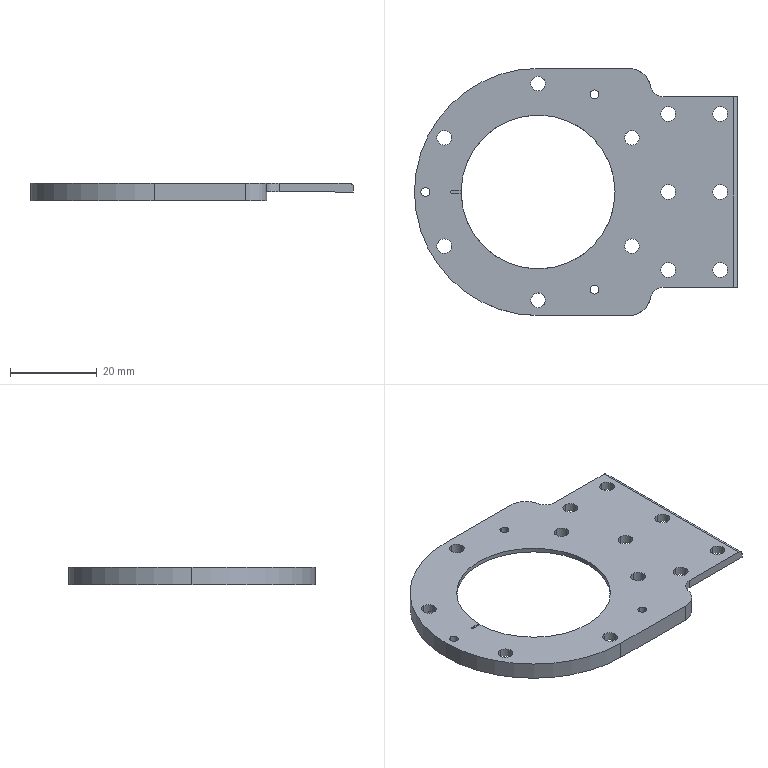NC program | NX | posted with a generic post | part box 74.5 x 57 x 4 mm
Lines 1635 to 1908 of 1908:
(PLANAR_MILL_2_COPY_COPY , TOOL : D6A45)
N3244 T01 M6
N3246 G54
N3248 G17 G0 G90 X33.045 Y22.642 S9500 M3
N3250 G43 Z30. H1
N3252 Z0.
N3254 G94 G1 X32.908 Z-0.037 F1250.
N3256 X32.875 Y22.608 Z-0.049
N3258 X32.908 Y22.392 Z-0.111
N3260 X33.125 Y22.425 Z-0.173
N3262 X33.092 Y22.642 Z-0.234
N3264 X32.875 Y22.608 Z-0.296
N3266 X32.908 Y22.392 Z-0.358
N3268 X33.125 Y22.425 Z-0.42
N3270 X33.092 Y22.642 Z-0.481
N3272 X32.875 Y22.608 Z-0.543
N3274 X32.908 Y22.392 Z-0.605
N3276 X33.125 Y22.425 Z-0.667
N3278 X33.092 Y22.642 Z-0.728
N3280 X32.875 Y22.608 Z-0.79
N3282 X32.908 Y22.392 Z-0.852
N3284 X33.125 Y22.425 Z-0.914
N3286 X33.092 Y22.642 Z-0.975
N3288 X33. Z-1.
N3290 G3 X32.875 Y22.517 R0.125
N3292 X33. Y22.642 R-0.125
N3294 G1 Z0.
N3296 G0 Z30.
N3298 X18.6 Y-0.866
N3300 Z0.
N3302 G1 Z-1.
N3304 G3 X19.1 Y0. R1.
N3306 G1 Y23.5
N3308 G2 X25. Y29.4 R5.9
N3310 G1 X46.
N3312 G2 X75.4 Y0. R29.4
N3314 X46. Y-29.4 R29.4
N3316 G1 X25.
N3318 G2 X19.1 Y-23.5 R5.9
N3320 G1 Y0.
N3322 G3 X18.6 Y0.866 R1.
N3324 G1 Z0.
N3326 G0 Z30.
N3328 X32.955 Y-22.642
N3330 Z0.
N3332 G1 X33.092 Z-0.037
N3334 X33.125 Y-22.608 Z-0.049
N3336 X33.092 Y-22.392 Z-0.111
N3338 X32.875 Y-22.425 Z-0.173
N3340 X32.908 Y-22.642 Z-0.234
N3342 X33.125 Y-22.608 Z-0.296
N3344 X33.092 Y-22.392 Z-0.358
N3346 X32.875 Y-22.425 Z-0.42
N3348 X32.908 Y-22.642 Z-0.481
N3350 X33.125 Y-22.608 Z-0.543
N3352 X33.092 Y-22.392 Z-0.605
N3354 X32.875 Y-22.425 Z-0.667
N3356 X32.908 Y-22.642 Z-0.728
N3358 X33.125 Y-22.608 Z-0.79
N3360 X33.092 Y-22.392 Z-0.852
N3362 X32.875 Y-22.425 Z-0.914
N3364 X32.908 Y-22.642 Z-0.975
N3366 X33. Z-1.
N3368 G3 X33.125 Y-22.517 R0.125
N3370 X33. Y-22.642 R-0.125
N3372 G1 Z0.
N3374 G0 Z30.
N3376 X34.2 Y-18.706
N3378 Z0.
N3380 G1 Z-1.
N3382 G3 X34.7 Y-19.572 R1.
N3384 X43.581 Y-22.47 R22.6
N3386 G2 X45.223 Y-24.81 R1.9
N3388 G3 X46.777 Y-24.81 R-0.8
N3390 G2 X48.419 Y-22.47 R1.9
N3392 G3 X64.25 Y-13.33 R22.6
N3394 G2 X67.098 Y-13.078 R1.9
N3396 G3 X67.875 Y-11.732 R-0.8
N3398 G2 X66.669 Y-9.14 R1.9
N3400 G3 X66.669 Y9.14 R22.6
N3402 G2 X67.875 Y11.732 R1.9
N3404 G3 X67.098 Y13.078 R-0.8
N3406 G2 X64.25 Y13.33 R1.9
N3408 G3 X48.419 Y22.47 R22.6
N3410 G2 X46.777 Y24.81 R1.9
N3412 G3 X45.223 Y24.81 R-0.8
N3414 G2 X43.581 Y22.47 R1.9
N3416 G3 X27.75 Y13.33 R22.6
N3418 G2 X24.902 Y13.078 R1.9
N3420 G3 X24.125 Y11.732 R-0.8
N3422 G2 X25.331 Y9.14 R1.9
N3424 G3 X25.331 Y-9.14 R22.6
N3426 G2 X24.125 Y-11.732 R1.9
N3428 G3 X24.902 Y-13.078 R-0.8
N3430 G2 X27.75 Y-13.33 R1.9
N3432 G3 X34.7 Y-19.572 R22.6
N3434 X35.7 Y-19.572 R1.
N3436 G1 Z0.
N3438 G0 Z30.
N3440 X72.125 Y-0.045
N3442 Z0.
N3444 G1 Y0.092 Z-0.037
N3446 X72.092 Y0.125 Z-0.049
N3448 X71.875 Y0.092 Z-0.111
N3450 X71.908 Y-0.125 Z-0.173
N3452 X72.125 Y-0.092 Z-0.234
N3454 X72.092 Y0.125 Z-0.296
N3456 X71.875 Y0.092 Z-0.358
N3458 X71.908 Y-0.125 Z-0.42
N3460 X72.125 Y-0.092 Z-0.481
N3462 X72.092 Y0.125 Z-0.543
N3464 X71.875 Y0.092 Z-0.605
N3466 X71.908 Y-0.125 Z-0.667
N3468 X72.125 Y-0.092 Z-0.728
N3470 X72.092 Y0.125 Z-0.79
N3472 X71.875 Y0.092 Z-0.852
N3474 X71.908 Y-0.125 Z-0.914
N3476 X72.125 Y-0.092 Z-0.975
N3478 Y0. Z-1.
N3480 G3 X72. Y0.125 R0.125
N3482 X72.125 Y0. R-0.125
N3484 G1 Z0.
N3486 G0 Z30.
(PLANAR_MILL_2_COPY_COPY_COPY , TOOL : D6A45)
N3488 X4.135 Y17.2
N3490 Z-2.
N3492 G1 X4.221 Z-2.023
N3494 X4.587 Y17.413 Z-2.137
N3496 X4.8 Y17.779 Z-2.25
N3498 Y18.221 Z-2.369
N3500 X4.587 Y18.587 Z-2.482
N3502 X4.221 Y18.8 Z-2.595
N3504 X3.779 Z-2.714
N3506 X3.413 Y18.587 Z-2.827
N3508 X3.2 Y18.221 Z-2.941
N3510 Y18. Z-3.
N3512 G3 X4. Y17.2 R0.8
N3514 X3.2 Y18. R-0.8
N3516 X3.45 Y17.567 R0.5
N3518 G1 Z-2.
N3520 G0 Z30.
N3522 X16.465 Y17.348
N3524 Z-2.
N3526 G1 X16.5 Y17.376 Z-2.012
N3528 X16.327 Y17.237 Z-2.071
N3530 X16.221 Y17.2 Z-2.101
N3532 X15.779 Z-2.22
N3534 X15.413 Y17.413 Z-2.333
N3536 X15.2 Y17.779 Z-2.447
N3538 Y18. Z-2.506
N3540 Y18.221 Z-2.565
N3542 X15.413 Y18.587 Z-2.679
N3544 X15.779 Y18.8 Z-2.792
N3546 X16. Z-2.851
N3548 X16.221 Z-2.911
N3550 X16.327 Y18.763 Z-2.941
N3552 X16.5 Y18.625 Z-3.
N3554 G3 X16.5 Y17.376 R-0.8
N3556 X16. Y18.242 R1.
N3558 G1 Z-2.
N3560 G0 Z30.
N3562 X16.465 Y-0.652
N3564 Z-2.
N3566 G1 X16.5 Y-0.625 Z-2.012
N3568 X16.327 Y-0.763 Z-2.071
N3570 X16.221 Y-0.8 Z-2.101
N3572 X16. Z-2.161
N3574 X15.779 Z-2.22
N3576 X15.413 Y-0.587 Z-2.333
N3578 X15.2 Y-0.221 Z-2.447
N3580 Y0.221 Z-2.565
N3582 X15.413 Y0.587 Z-2.679
N3584 X15.779 Y0.8 Z-2.792
N3586 X16. Z-2.851
N3588 X16.221 Z-2.911
N3590 X16.327 Y0.763 Z-2.941
N3592 X16.5 Y0.625 Z-3.
N3594 G3 X16.5 Y-0.625 R-0.8
N3596 X16. Y0.242 R1.
N3598 G1 Z-2.
N3600 G0 Z30.
N3602 X4.135 Y-0.8
N3604 Z-2.
N3606 G1 X4.221 Z-2.023
N3608 X4.587 Y-0.587 Z-2.137
N3610 X4.8 Y-0.221 Z-2.25
N3612 Y0.221 Z-2.369
N3614 X4.587 Y0.587 Z-2.482
N3616 X4.221 Y0.8 Z-2.595
N3618 X3.779 Z-2.714
N3620 X3.413 Y0.587 Z-2.827
N3622 X3.2 Y0.221 Z-2.941
N3624 Y0. Z-3.
N3626 G3 X4. Y-0.8 R0.8
N3628 X3.2 Y0. R-0.8
N3630 X3.45 Y-0.433 R0.5
N3632 G1 Z-2.
N3634 G0 Z30.
N3636 X4.135 Y-18.8
N3638 Z-2.
N3640 G1 X4.221 Z-2.023
N3642 X4.587 Y-18.587 Z-2.137
N3644 X4.8 Y-18.221 Z-2.25
N3646 Y-17.779 Z-2.369
N3648 X4.587 Y-17.413 Z-2.482
N3650 X4.221 Y-17.2 Z-2.595
N3652 X3.779 Z-2.714
N3654 X3.413 Y-17.413 Z-2.827
N3656 X3.2 Y-17.779 Z-2.941
N3658 Y-18. Z-3.
N3660 G3 X4. Y-18.8 R0.8
N3662 X3.2 Y-18. R-0.8
N3664 X3.45 Y-18.433 R0.5
N3666 G1 Z-2.
N3668 G0 Z30.
N3670 X16.465 Y-18.652
N3672 Z-2.
N3674 G1 X16.5 Y-18.625 Z-2.012
N3676 X16.327 Y-18.763 Z-2.071
N3678 X16.221 Y-18.8 Z-2.101
N3680 X15.779 Z-2.22
N3682 X15.413 Y-18.587 Z-2.333
N3684 X15.2 Y-18.221 Z-2.447
N3686 Y-18. Z-2.506
N3688 Y-17.779 Z-2.565
N3690 X15.413 Y-17.413 Z-2.679
N3692 X15.779 Y-17.2 Z-2.792
N3694 X16. Z-2.851
N3696 X16.221 Z-2.911
N3698 X16.327 Y-17.237 Z-2.941
N3700 X16.5 Y-17.376 Z-3.
N3702 G3 X16.5 Y-18.625 R-0.8
N3704 X16. Y-17.758 R1.
N3706 G1 Z-2.
N3708 G0 Z30.
N3710 X15.322 Y-24.157
N3712 Z-2.
N3714 G1 Z-3.
N3716 X16. Y-23.766
N3718 G3 X16.5 Y-22.9 R1.
N3720 G1 X0.1
N3722 G2 X-0.9 Y-21.9 R1.
N3724 G1 Y21.9
N3726 G2 X0.1 Y22.9 R1.
N3728 G1 X16.5
N3730 G3 X16. Y23.766 R1.
N3732 G1 X15.322 Y24.157
N3734 Z-2.
N3736 G0 Z30.
N3738 M5
(PLANAR_MILL , TOOL : D4)
N3740 T11 M6
N3742 G54
N3744 G17 G0 G90 X44.408 Y-20.951 S9500 M3
N3746 G43 Z30. H11
N3748 Z-1.
N3750 G94 G1 Z-2. F1250.
N3752 G41 X44.448 Y-21.043 D11
N3754 G3 X45.245 Y-21.487 R1.
N3756 X67.487 Y-0.755 R21.5
N3758 X45.245 Y-21.487 R-21.5
N3760 X46.07 Y-21.1 R1.
N3762 G40
N3764 G1 X46.117 Y-21.011
N3766 Z-1.
N3768 G0 Z30.
N3770 M5
N3772 M2